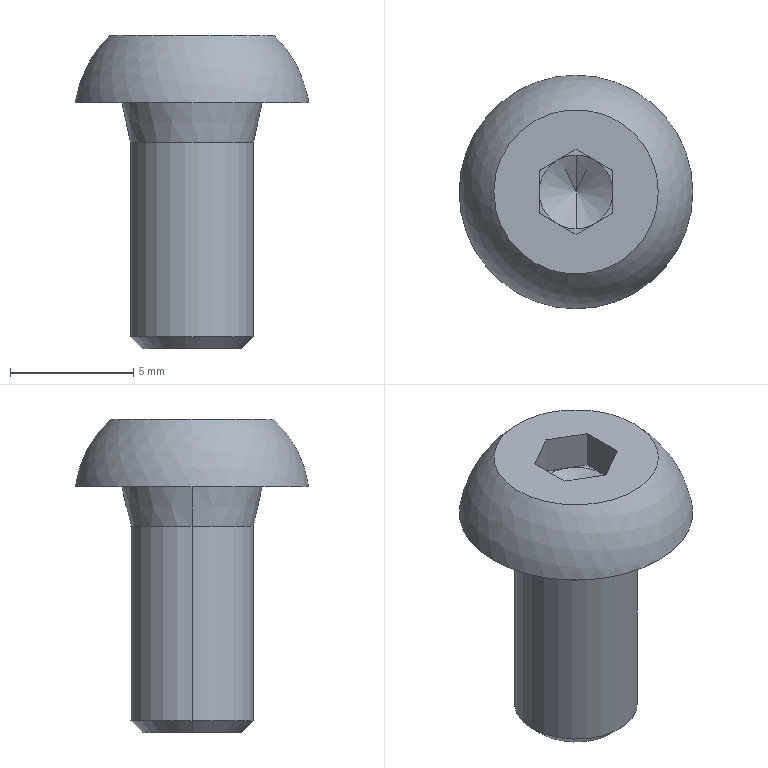Part | SolidWorks | features BaseBody 1 | 1 solid | 24 faces | box 9.5 x 9.5 x 12.75 mm | volume 341.504 mm3 | plane 15 | cone 6 | cylinder 2 | sphere 1 | commonest cylinder face diameters 5 x2
STEP:
#1=CARTESIAN_POINT('',(2.5,0.,0.));
#2=VERTEX_POINT('',#1);
#3=CARTESIAN_POINT('',(-2.5,0.,0.));
#4=VERTEX_POINT('',#3);
#5=CARTESIAN_POINT('',(0.,0.,0.));
#6=DIRECTION('',(0.,0.,1.));
#7=DIRECTION('',(1.,0.,0.));
#8=AXIS2_PLACEMENT_3D('',#5,#6,#7);
#9=CIRCLE('',#8,2.5);
#10=EDGE_CURVE('',#2,#4,#9,.T.);
#11=ORIENTED_EDGE('',*,*,#10,.T.);
#12=CARTESIAN_POINT('',(-2.85,0.,1.6));
#13=VERTEX_POINT('',#12);
#14=CARTESIAN_POINT('',(-2.85,0.,1.6));
#15=DIRECTION('',(-0.2137,0.,0.9769));
#16=VECTOR('',#15,1000.);
#17=LINE('',#14,#16);
#18=EDGE_CURVE('',#4,#13,#17,.T.);
#19=ORIENTED_EDGE('',*,*,#18,.T.);
#20=CARTESIAN_POINT('',(2.85,0.,1.6));
#21=VERTEX_POINT('',#20);
#22=CARTESIAN_POINT('',(0.,0.,1.6));
#23=DIRECTION('',(0.,0.,-1.));
#24=DIRECTION('',(1.,0.,0.));
#25=AXIS2_PLACEMENT_3D('',#22,#23,#24);
#26=CIRCLE('',#25,2.85);
#27=EDGE_CURVE('',#13,#21,#26,.T.);
#28=ORIENTED_EDGE('',*,*,#27,.T.);
#29=CARTESIAN_POINT('',(2.85,0.,1.6));
#30=DIRECTION('',(0.2137,0.,0.9769));
#31=VECTOR('',#30,1000.);
#32=LINE('',#29,#31);
#33=EDGE_CURVE('',#2,#21,#32,.T.);
#34=ORIENTED_EDGE('',*,*,#33,.F.);
#35=EDGE_LOOP('',(#11,#19,#28,#34));
#36=FACE_OUTER_BOUND('',#35,.T.);
#37=CARTESIAN_POINT('',(0.,0.,1.6));
#38=DIRECTION('',(0.,0.,1.));
#39=DIRECTION('',(1.,0.,0.));
#40=AXIS2_PLACEMENT_3D('',#37,#38,#39);
#41=CONICAL_SURFACE('',#40,2.85,0.2154);
#42=ADVANCED_FACE('',(#36),#41,.T.);
#43=CARTESIAN_POINT('',(2.5,0.,-7.91));
#44=VERTEX_POINT('',#43);
#45=CARTESIAN_POINT('',(-2.5,0.,-7.91));
#46=VERTEX_POINT('',#45);
#47=CARTESIAN_POINT('',(0.,0.,-7.91));
#48=DIRECTION('',(0.,0.,1.));
#49=DIRECTION('',(1.,0.,0.));
#50=AXIS2_PLACEMENT_3D('',#47,#48,#49);
#51=CIRCLE('',#50,2.5);
#52=EDGE_CURVE('',#44,#46,#51,.T.);
#53=ORIENTED_EDGE('',*,*,#52,.T.);
#54=CARTESIAN_POINT('',(-2.5,0.,-8.4));
#55=DIRECTION('',(0.,0.,1.));
#56=VECTOR('',#55,1000.);
#57=LINE('',#54,#56);
#58=EDGE_CURVE('',#46,#4,#57,.T.);
#59=ORIENTED_EDGE('',*,*,#58,.T.);
#60=ORIENTED_EDGE('',*,*,#10,.F.);
#61=CARTESIAN_POINT('',(2.5,0.,-8.4));
#62=DIRECTION('',(0.,0.,1.));
#63=VECTOR('',#62,1000.);
#64=LINE('',#61,#63);
#65=EDGE_CURVE('',#44,#2,#64,.T.);
#66=ORIENTED_EDGE('',*,*,#65,.F.);
#67=EDGE_LOOP('',(#53,#59,#60,#66));
#68=FACE_OUTER_BOUND('',#67,.T.);
#69=CARTESIAN_POINT('',(0.,0.,-8.4));
#70=DIRECTION('',(0.,0.,1.));
#71=DIRECTION('',(1.,0.,0.));
#72=AXIS2_PLACEMENT_3D('',#69,#70,#71);
#73=CYLINDRICAL_SURFACE('',#72,2.5);
#74=ADVANCED_FACE('',(#68),#73,.T.);
#75=CARTESIAN_POINT('',(0.,0.,1.924));
#76=VERTEX_POINT('',#75);
#77=CARTESIAN_POINT('',(0.,-1.5,2.79));
#78=VERTEX_POINT('',#77);
#79=CARTESIAN_POINT('',(0.,-1.5,2.79));
#80=DIRECTION('',(0.,-0.866,0.5));
#81=VECTOR('',#80,1000.);
#82=LINE('',#79,#81);
#83=EDGE_CURVE('',#76,#78,#82,.T.);
#84=ORIENTED_EDGE('',*,*,#83,.F.);
#85=CARTESIAN_POINT('',(0.,1.5,2.79));
#86=VERTEX_POINT('',#85);
#87=CARTESIAN_POINT('',(0.,1.5,2.79));
#88=DIRECTION('',(0.,0.866,0.5));
#89=VECTOR('',#88,1000.);
#90=LINE('',#87,#89);
#91=EDGE_CURVE('',#76,#86,#90,.T.);
#92=ORIENTED_EDGE('',*,*,#91,.T.);
#93=CARTESIAN_POINT('',(-0.75,1.299,2.79));
#94=VERTEX_POINT('',#93);
#95=CARTESIAN_POINT('',(0.,0.,2.79));
#96=DIRECTION('',(0.,0.,-1.));
#97=DIRECTION('',(0.,-1.,0.));
#98=AXIS2_PLACEMENT_3D('',#95,#96,#97);
#99=CIRCLE('',#98,1.5);
#100=EDGE_CURVE('',#94,#86,#99,.T.);
#101=ORIENTED_EDGE('',*,*,#100,.F.);
#102=CARTESIAN_POINT('',(-1.5,0.,2.79));
#103=VERTEX_POINT('',#102);
#104=CARTESIAN_POINT('',(0.,0.,2.79));
#105=DIRECTION('',(0.,0.,-1.));
#106=DIRECTION('',(0.,-1.,0.));
#107=AXIS2_PLACEMENT_3D('',#104,#105,#106);
#108=CIRCLE('',#107,1.5);
#109=EDGE_CURVE('',#103,#94,#108,.T.);
#110=ORIENTED_EDGE('',*,*,#109,.F.);
#111=CARTESIAN_POINT('',(-0.75,-1.299,2.79));
#112=VERTEX_POINT('',#111);
#113=CARTESIAN_POINT('',(0.,0.,2.79));
#114=DIRECTION('',(0.,0.,-1.));
#115=DIRECTION('',(0.,-1.,0.));
#116=AXIS2_PLACEMENT_3D('',#113,#114,#115);
#117=CIRCLE('',#116,1.5);
#118=EDGE_CURVE('',#112,#103,#117,.T.);
#119=ORIENTED_EDGE('',*,*,#118,.F.);
#120=CARTESIAN_POINT('',(0.,0.,2.79));
#121=DIRECTION('',(0.,0.,-1.));
#122=DIRECTION('',(0.,-1.,0.));
#123=AXIS2_PLACEMENT_3D('',#120,#121,#122);
#124=CIRCLE('',#123,1.5);
#125=EDGE_CURVE('',#78,#112,#124,.T.);
#126=ORIENTED_EDGE('',*,*,#125,.F.);
#127=EDGE_LOOP('',(#84,#92,#101,#110,#119,#126));
#128=FACE_OUTER_BOUND('',#127,.T.);
#129=CARTESIAN_POINT('',(0.,0.,2.79));
#130=DIRECTION('',(0.,0.,1.));
#131=DIRECTION('',(0.,-1.,0.));
#132=AXIS2_PLACEMENT_3D('',#129,#130,#131);
#133=CONICAL_SURFACE('',#132,1.5,1.047);
#134=ADVANCED_FACE('',(#128),#133,.F.);
#135=CARTESIAN_POINT('',(2.01,0.,-8.4));
#136=VERTEX_POINT('',#135);
#137=CARTESIAN_POINT('',(-2.01,0.,-8.4));
#138=VERTEX_POINT('',#137);
#139=CARTESIAN_POINT('',(0.,0.,-8.4));
#140=DIRECTION('',(0.,0.,1.));
#141=DIRECTION('',(1.,0.,0.));
#142=AXIS2_PLACEMENT_3D('',#139,#140,#141);
#143=CIRCLE('',#142,2.01);
#144=EDGE_CURVE('',#136,#138,#143,.T.);
#145=ORIENTED_EDGE('',*,*,#144,.T.);
#146=CARTESIAN_POINT('',(-2.5,0.,-7.91));
#147=DIRECTION('',(-0.7071,0.,0.7071));
#148=VECTOR('',#147,1000.);
#149=LINE('',#146,#148);
#150=EDGE_CURVE('',#138,#46,#149,.T.);
#151=ORIENTED_EDGE('',*,*,#150,.T.);
#152=ORIENTED_EDGE('',*,*,#52,.F.);
#153=CARTESIAN_POINT('',(2.5,0.,-7.91));
#154=DIRECTION('',(0.7071,0.,0.7071));
#155=VECTOR('',#154,1000.);
#156=LINE('',#153,#155);
#157=EDGE_CURVE('',#136,#44,#156,.T.);
#158=ORIENTED_EDGE('',*,*,#157,.F.);
#159=EDGE_LOOP('',(#145,#151,#152,#158));
#160=FACE_OUTER_BOUND('',#159,.T.);
#161=CARTESIAN_POINT('',(0.,0.,-7.91));
#162=DIRECTION('',(0.,0.,1.));
#163=DIRECTION('',(1.,0.,0.));
#164=AXIS2_PLACEMENT_3D('',#161,#162,#163);
#165=CONICAL_SURFACE('',#164,2.5,0.7854);
#166=ADVANCED_FACE('',(#160),#165,.T.);
#167=CARTESIAN_POINT('',(-3.339,0.,4.35));
#168=VERTEX_POINT('',#167);
#169=CARTESIAN_POINT('',(3.339,0.,4.35));
#170=VERTEX_POINT('',#169);
#171=CARTESIAN_POINT('',(0.,0.,4.35));
#172=DIRECTION('',(0.,0.,-1.));
#173=DIRECTION('',(-1.,0.,0.));
#174=AXIS2_PLACEMENT_3D('',#171,#172,#173);
#175=CIRCLE('',#174,3.339);
#176=EDGE_CURVE('',#168,#170,#175,.T.);
#177=ORIENTED_EDGE('',*,*,#176,.T.);
#178=CARTESIAN_POINT('',(0.,0.,4.35));
#179=DIRECTION('',(0.,0.,-1.));
#180=DIRECTION('',(-1.,0.,0.));
#181=AXIS2_PLACEMENT_3D('',#178,#179,#180);
#182=CIRCLE('',#181,3.339);
#183=EDGE_CURVE('',#170,#168,#182,.T.);
#184=ORIENTED_EDGE('',*,*,#183,.T.);
#185=EDGE_LOOP('',(#177,#184));
#186=FACE_BOUND('',#185,.T.);
#187=CARTESIAN_POINT('',(4.75,0.,1.6));
#188=VERTEX_POINT('',#187);
#189=CARTESIAN_POINT('',(-4.75,0.,1.6));
#190=VERTEX_POINT('',#189);
#191=CARTESIAN_POINT('',(0.,0.,1.6));
#192=DIRECTION('',(0.,0.,1.));
#193=DIRECTION('',(1.,0.,0.));
#194=AXIS2_PLACEMENT_3D('',#191,#192,#193);
#195=CIRCLE('',#194,4.75);
#196=EDGE_CURVE('',#188,#190,#195,.T.);
#197=ORIENTED_EDGE('',*,*,#196,.T.);
#198=CARTESIAN_POINT('',(0.,0.,1.6));
#199=DIRECTION('',(0.,0.,1.));
#200=DIRECTION('',(1.,0.,0.));
#201=AXIS2_PLACEMENT_3D('',#198,#199,#200);
#202=CIRCLE('',#201,4.75);
#203=EDGE_CURVE('',#190,#188,#202,.T.);
#204=ORIENTED_EDGE('',*,*,#203,.T.);
#205=EDGE_LOOP('',(#197,#204));
#206=FACE_OUTER_BOUND('',#205,.T.);
#207=CARTESIAN_POINT('',(0.,0.,0.9));
#208=DIRECTION('',(0.1289,0.,0.9917));
#209=DIRECTION('',(-0.9917,0.,0.1289));
#210=AXIS2_PLACEMENT_3D('',#207,#208,#209);
#211=SPHERICAL_SURFACE('',#210,4.801);
#212=ADVANCED_FACE('',(#186,#206),#211,.T.);
#213=ORIENTED_EDGE('',*,*,#176,.F.);
#214=ORIENTED_EDGE('',*,*,#183,.F.);
#215=EDGE_LOOP('',(#213,#214));
#216=FACE_OUTER_BOUND('',#215,.T.);
#217=CARTESIAN_POINT('',(0.,-1.732,4.35));
#218=VERTEX_POINT('',#217);
#219=CARTESIAN_POINT('',(1.5,-0.866,4.35));
#220=VERTEX_POINT('',#219);
#221=CARTESIAN_POINT('',(0.,-1.732,4.35));
#222=DIRECTION('',(0.866,0.5,0.));
#223=VECTOR('',#222,1000.);
#224=LINE('',#221,#223);
#225=EDGE_CURVE('',#218,#220,#224,.T.);
#226=ORIENTED_EDGE('',*,*,#225,.F.);
#227=CARTESIAN_POINT('',(-1.5,-0.866,4.35));
#228=VERTEX_POINT('',#227);
#229=CARTESIAN_POINT('',(-1.5,-0.866,4.35));
#230=DIRECTION('',(0.866,-0.5,0.));
#231=VECTOR('',#230,1000.);
#232=LINE('',#229,#231);
#233=EDGE_CURVE('',#228,#218,#232,.T.);
#234=ORIENTED_EDGE('',*,*,#233,.F.);
#235=CARTESIAN_POINT('',(-1.5,0.866,4.35));
#236=VERTEX_POINT('',#235);
#237=CARTESIAN_POINT('',(-1.5,0.,4.35));
#238=DIRECTION('',(0.,-1.,0.));
#239=VECTOR('',#238,1000.);
#240=LINE('',#237,#239);
#241=EDGE_CURVE('',#236,#228,#240,.T.);
#242=ORIENTED_EDGE('',*,*,#241,.F.);
#243=CARTESIAN_POINT('',(0.,1.732,4.35));
#244=VERTEX_POINT('',#243);
#245=CARTESIAN_POINT('',(0.,1.732,4.35));
#246=DIRECTION('',(-0.866,-0.5,0.));
#247=VECTOR('',#246,1000.);
#248=LINE('',#245,#247);
#249=EDGE_CURVE('',#244,#236,#248,.T.);
#250=ORIENTED_EDGE('',*,*,#249,.F.);
#251=CARTESIAN_POINT('',(1.5,0.866,4.35));
#252=VERTEX_POINT('',#251);
#253=CARTESIAN_POINT('',(1.5,0.866,4.35));
#254=DIRECTION('',(-0.866,0.5,0.));
#255=VECTOR('',#254,1000.);
#256=LINE('',#253,#255);
#257=EDGE_CURVE('',#252,#244,#256,.T.);
#258=ORIENTED_EDGE('',*,*,#257,.F.);
#259=CARTESIAN_POINT('',(1.5,0.,4.35));
#260=DIRECTION('',(0.,1.,0.));
#261=VECTOR('',#260,1000.);
#262=LINE('',#259,#261);
#263=EDGE_CURVE('',#220,#252,#262,.T.);
#264=ORIENTED_EDGE('',*,*,#263,.F.);
#265=EDGE_LOOP('',(#226,#234,#242,#250,#258,#264));
#266=FACE_BOUND('',#265,.T.);
#267=CARTESIAN_POINT('',(0.,0.,4.35));
#268=DIRECTION('',(0.,0.,-1.));
#269=DIRECTION('',(-1.,0.,0.));
#270=AXIS2_PLACEMENT_3D('',#267,#268,#269);
#271=PLANE('',#270);
#272=ADVANCED_FACE('',(#216,#266),#271,.F.);
#273=ORIENTED_EDGE('',*,*,#196,.F.);
#274=ORIENTED_EDGE('',*,*,#203,.F.);
#275=EDGE_LOOP('',(#273,#274));
#276=FACE_OUTER_BOUND('',#275,.T.);
#277=CARTESIAN_POINT('',(0.,0.,1.6));
#278=DIRECTION('',(0.,0.,-1.));
#279=DIRECTION('',(1.,0.,0.));
#280=AXIS2_PLACEMENT_3D('',#277,#278,#279);
#281=CIRCLE('',#280,2.85);
#282=EDGE_CURVE('',#21,#13,#281,.T.);
#283=ORIENTED_EDGE('',*,*,#282,.F.);
#284=ORIENTED_EDGE('',*,*,#27,.F.);
#285=EDGE_LOOP('',(#283,#284));
#286=FACE_BOUND('',#285,.T.);
#287=CARTESIAN_POINT('',(0.,4.75,1.6));
#288=DIRECTION('',(0.,0.,1.));
#289=DIRECTION('',(1.,0.,0.));
#290=AXIS2_PLACEMENT_3D('',#287,#288,#289);
#291=PLANE('',#290);
#292=ADVANCED_FACE('',(#276,#286),#291,.F.);
#293=CARTESIAN_POINT('',(1.5,0.866,2.79));
#294=VERTEX_POINT('',#293);
#295=CARTESIAN_POINT('',(1.5,0.866,2.79));
#296=DIRECTION('',(0.,0.,1.));
#297=VECTOR('',#296,1000.);
#298=LINE('',#295,#297);
#299=EDGE_CURVE('',#294,#252,#298,.T.);
#300=ORIENTED_EDGE('',*,*,#299,.F.);
#301=CARTESIAN_POINT('',(1.5,0.,2.79));
#302=VERTEX_POINT('',#301);
#303=CARTESIAN_POINT('',(1.5,-0.866,2.79));
#304=DIRECTION('',(0.,1.,0.));
#305=VECTOR('',#304,1000.);
#306=LINE('',#303,#305);
#307=EDGE_CURVE('',#302,#294,#306,.T.);
#308=ORIENTED_EDGE('',*,*,#307,.F.);
#309=CARTESIAN_POINT('',(1.5,-0.866,2.79));
#310=VERTEX_POINT('',#309);
#311=CARTESIAN_POINT('',(1.5,-0.866,2.79));
#312=DIRECTION('',(0.,1.,0.));
#313=VECTOR('',#312,1000.);
#314=LINE('',#311,#313);
#315=EDGE_CURVE('',#310,#302,#314,.T.);
#316=ORIENTED_EDGE('',*,*,#315,.F.);
#317=CARTESIAN_POINT('',(1.5,-0.866,2.79));
#318=DIRECTION('',(0.,0.,-1.));
#319=VECTOR('',#318,1000.);
#320=LINE('',#317,#319);
#321=EDGE_CURVE('',#220,#310,#320,.T.);
#322=ORIENTED_EDGE('',*,*,#321,.F.);
#323=ORIENTED_EDGE('',*,*,#263,.T.);
#324=EDGE_LOOP('',(#300,#308,#316,#322,#323));
#325=FACE_OUTER_BOUND('',#324,.T.);
#326=CARTESIAN_POINT('',(1.5,-0.866,2.79));
#327=DIRECTION('',(1.,0.,0.));
#328=DIRECTION('',(0.,0.,-1.));
#329=AXIS2_PLACEMENT_3D('',#326,#327,#328);
#330=PLANE('',#329);
#331=ADVANCED_FACE('',(#325),#330,.F.);
#332=ORIENTED_EDGE('',*,*,#321,.T.);
#333=CARTESIAN_POINT('',(0.75,-1.299,2.79));
#334=VERTEX_POINT('',#333);
#335=CARTESIAN_POINT('',(0.,-1.732,2.79));
#336=DIRECTION('',(0.866,0.5,0.));
#337=VECTOR('',#336,1000.);
#338=LINE('',#335,#337);
#339=EDGE_CURVE('',#334,#310,#338,.T.);
#340=ORIENTED_EDGE('',*,*,#339,.F.);
#341=CARTESIAN_POINT('',(0.,-1.732,2.79));
#342=VERTEX_POINT('',#341);
#343=CARTESIAN_POINT('',(0.,-1.732,2.79));
#344=DIRECTION('',(0.866,0.5,0.));
#345=VECTOR('',#344,1000.);
#346=LINE('',#343,#345);
#347=EDGE_CURVE('',#342,#334,#346,.T.);
#348=ORIENTED_EDGE('',*,*,#347,.F.);
#349=CARTESIAN_POINT('',(0.,-1.732,2.79));
#350=DIRECTION('',(0.,0.,-1.));
#351=VECTOR('',#350,1000.);
#352=LINE('',#349,#351);
#353=EDGE_CURVE('',#218,#342,#352,.T.);
#354=ORIENTED_EDGE('',*,*,#353,.F.);
#355=ORIENTED_EDGE('',*,*,#225,.T.);
#356=EDGE_LOOP('',(#332,#340,#348,#354,#355));
#357=FACE_OUTER_BOUND('',#356,.T.);
#358=CARTESIAN_POINT('',(0.,-1.732,2.79));
#359=DIRECTION('',(0.5,-0.866,0.));
#360=DIRECTION('',(0.866,0.5,0.));
#361=AXIS2_PLACEMENT_3D('',#358,#359,#360);
#362=PLANE('',#361);
#363=ADVANCED_FACE('',(#357),#362,.F.);
#364=ORIENTED_EDGE('',*,*,#353,.T.);
#365=CARTESIAN_POINT('',(-1.5,-0.866,2.79));
#366=DIRECTION('',(0.866,-0.5,0.));
#367=VECTOR('',#366,1000.);
#368=LINE('',#365,#367);
#369=EDGE_CURVE('',#112,#342,#368,.T.);
#370=ORIENTED_EDGE('',*,*,#369,.F.);
#371=CARTESIAN_POINT('',(-1.5,-0.866,2.79));
#372=VERTEX_POINT('',#371);
#373=CARTESIAN_POINT('',(-1.5,-0.866,2.79));
#374=DIRECTION('',(0.866,-0.5,0.));
#375=VECTOR('',#374,1000.);
#376=LINE('',#373,#375);
#377=EDGE_CURVE('',#372,#112,#376,.T.);
#378=ORIENTED_EDGE('',*,*,#377,.F.);
#379=CARTESIAN_POINT('',(-1.5,-0.866,2.79));
#380=DIRECTION('',(0.,0.,-1.));
#381=VECTOR('',#380,1000.);
#382=LINE('',#379,#381);
#383=EDGE_CURVE('',#228,#372,#382,.T.);
#384=ORIENTED_EDGE('',*,*,#383,.F.);
#385=ORIENTED_EDGE('',*,*,#233,.T.);
#386=EDGE_LOOP('',(#364,#370,#378,#384,#385));
#387=FACE_OUTER_BOUND('',#386,.T.);
#388=CARTESIAN_POINT('',(-1.5,-0.866,2.79));
#389=DIRECTION('',(-0.5,-0.866,0.));
#390=DIRECTION('',(0.866,-0.5,0.));
#391=AXIS2_PLACEMENT_3D('',#388,#389,#390);
#392=PLANE('',#391);
#393=ADVANCED_FACE('',(#387),#392,.F.);
#394=ORIENTED_EDGE('',*,*,#383,.T.);
#395=CARTESIAN_POINT('',(-1.5,0.866,2.79));
#396=DIRECTION('',(0.,-1.,0.));
#397=VECTOR('',#396,1000.);
#398=LINE('',#395,#397);
#399=EDGE_CURVE('',#103,#372,#398,.T.);
#400=ORIENTED_EDGE('',*,*,#399,.F.);
#401=CARTESIAN_POINT('',(-1.5,0.866,2.79));
#402=VERTEX_POINT('',#401);
#403=CARTESIAN_POINT('',(-1.5,0.866,2.79));
#404=DIRECTION('',(0.,-1.,0.));
#405=VECTOR('',#404,1000.);
#406=LINE('',#403,#405);
#407=EDGE_CURVE('',#402,#103,#406,.T.);
#408=ORIENTED_EDGE('',*,*,#407,.F.);
#409=CARTESIAN_POINT('',(-1.5,0.866,2.79));
#410=DIRECTION('',(0.,0.,-1.));
#411=VECTOR('',#410,1000.);
#412=LINE('',#409,#411);
#413=EDGE_CURVE('',#236,#402,#412,.T.);
#414=ORIENTED_EDGE('',*,*,#413,.F.);
#415=ORIENTED_EDGE('',*,*,#241,.T.);
#416=EDGE_LOOP('',(#394,#400,#408,#414,#415));
#417=FACE_OUTER_BOUND('',#416,.T.);
#418=CARTESIAN_POINT('',(-1.5,0.866,2.79));
#419=DIRECTION('',(-1.,0.,0.));
#420=DIRECTION('',(0.,-1.,0.));
#421=AXIS2_PLACEMENT_3D('',#418,#419,#420);
#422=PLANE('',#421);
#423=ADVANCED_FACE('',(#417),#422,.F.);
#424=ORIENTED_EDGE('',*,*,#413,.T.);
#425=CARTESIAN_POINT('',(0.,1.732,2.79));
#426=DIRECTION('',(-0.866,-0.5,0.));
#427=VECTOR('',#426,1000.);
#428=LINE('',#425,#427);
#429=EDGE_CURVE('',#94,#402,#428,.T.);
#430=ORIENTED_EDGE('',*,*,#429,.F.);
#431=CARTESIAN_POINT('',(0.,1.732,2.79));
#432=VERTEX_POINT('',#431);
#433=CARTESIAN_POINT('',(0.,1.732,2.79));
#434=DIRECTION('',(-0.866,-0.5,0.));
#435=VECTOR('',#434,1000.);
#436=LINE('',#433,#435);
#437=EDGE_CURVE('',#432,#94,#436,.T.);
#438=ORIENTED_EDGE('',*,*,#437,.F.);
#439=CARTESIAN_POINT('',(0.,1.732,2.79));
#440=DIRECTION('',(0.,0.,-1.));
#441=VECTOR('',#440,1000.);
#442=LINE('',#439,#441);
#443=EDGE_CURVE('',#244,#432,#442,.T.);
#444=ORIENTED_EDGE('',*,*,#443,.F.);
#445=ORIENTED_EDGE('',*,*,#249,.T.);
#446=EDGE_LOOP('',(#424,#430,#438,#444,#445));
#447=FACE_OUTER_BOUND('',#446,.T.);
#448=CARTESIAN_POINT('',(0.,1.732,2.79));
#449=DIRECTION('',(-0.5,0.866,0.));
#450=DIRECTION('',(-0.866,-0.5,0.));
#451=AXIS2_PLACEMENT_3D('',#448,#449,#450);
#452=PLANE('',#451);
#453=ADVANCED_FACE('',(#447),#452,.F.);
#454=ORIENTED_EDGE('',*,*,#443,.T.);
#455=CARTESIAN_POINT('',(0.75,1.299,2.79));
#456=VERTEX_POINT('',#455);
#457=CARTESIAN_POINT('',(1.5,0.866,2.79));
#458=DIRECTION('',(-0.866,0.5,0.));
#459=VECTOR('',#458,1000.);
#460=LINE('',#457,#459);
#461=EDGE_CURVE('',#456,#432,#460,.T.);
#462=ORIENTED_EDGE('',*,*,#461,.F.);
#463=CARTESIAN_POINT('',(1.5,0.866,2.79));
#464=DIRECTION('',(-0.866,0.5,0.));
#465=VECTOR('',#464,1000.);
#466=LINE('',#463,#465);
#467=EDGE_CURVE('',#294,#456,#466,.T.);
#468=ORIENTED_EDGE('',*,*,#467,.F.);
#469=ORIENTED_EDGE('',*,*,#299,.T.);
#470=ORIENTED_EDGE('',*,*,#257,.T.);
#471=EDGE_LOOP('',(#454,#462,#468,#469,#470));
#472=FACE_OUTER_BOUND('',#471,.T.);
#473=CARTESIAN_POINT('',(1.5,0.866,2.79));
#474=DIRECTION('',(0.5,0.866,0.));
#475=DIRECTION('',(-0.866,0.5,0.));
#476=AXIS2_PLACEMENT_3D('',#473,#474,#475);
#477=PLANE('',#476);
#478=ADVANCED_FACE('',(#472),#477,.F.);
#479=ORIENTED_EDGE('',*,*,#18,.F.);
#480=CARTESIAN_POINT('',(0.,0.,0.));
#481=DIRECTION('',(0.,0.,1.));
#482=DIRECTION('',(1.,0.,0.));
#483=AXIS2_PLACEMENT_3D('',#480,#481,#482);
#484=CIRCLE('',#483,2.5);
#485=EDGE_CURVE('',#4,#2,#484,.T.);
#486=ORIENTED_EDGE('',*,*,#485,.T.);
#487=ORIENTED_EDGE('',*,*,#33,.T.);
#488=ORIENTED_EDGE('',*,*,#282,.T.);
#489=EDGE_LOOP('',(#479,#486,#487,#488));
#490=FACE_OUTER_BOUND('',#489,.T.);
#491=CARTESIAN_POINT('',(0.,0.,1.6));
#492=DIRECTION('',(0.,0.,1.));
#493=DIRECTION('',(1.,0.,0.));
#494=AXIS2_PLACEMENT_3D('',#491,#492,#493);
#495=CONICAL_SURFACE('',#494,2.85,0.2154);
#496=ADVANCED_FACE('',(#490),#495,.T.);
#497=CARTESIAN_POINT('',(0.,0.,2.79));
#498=DIRECTION('',(0.,0.,-1.));
#499=DIRECTION('',(0.,-1.,0.));
#500=AXIS2_PLACEMENT_3D('',#497,#498,#499);
#501=CIRCLE('',#500,1.5);
#502=EDGE_CURVE('',#456,#302,#501,.T.);
#503=ORIENTED_EDGE('',*,*,#502,.T.);
#504=ORIENTED_EDGE('',*,*,#307,.T.);
#505=ORIENTED_EDGE('',*,*,#467,.T.);
#506=EDGE_LOOP('',(#503,#504,#505));
#507=FACE_OUTER_BOUND('',#506,.T.);
#508=CARTESIAN_POINT('',(0.,0.,2.79));
#509=DIRECTION('',(0.,0.,1.));
#510=DIRECTION('',(1.,0.,0.));
#511=AXIS2_PLACEMENT_3D('',#508,#509,#510);
#512=PLANE('',#511);
#513=ADVANCED_FACE('',(#507),#512,.T.);
#514=CARTESIAN_POINT('',(0.,0.,2.79));
#515=DIRECTION('',(0.,0.,-1.));
#516=DIRECTION('',(0.,-1.,0.));
#517=AXIS2_PLACEMENT_3D('',#514,#515,#516);
#518=CIRCLE('',#517,1.5);
#519=EDGE_CURVE('',#302,#334,#518,.T.);
#520=ORIENTED_EDGE('',*,*,#519,.T.);
#521=ORIENTED_EDGE('',*,*,#339,.T.);
#522=ORIENTED_EDGE('',*,*,#315,.T.);
#523=EDGE_LOOP('',(#520,#521,#522));
#524=FACE_OUTER_BOUND('',#523,.T.);
#525=CARTESIAN_POINT('',(0.,0.,2.79));
#526=DIRECTION('',(0.,0.,1.));
#527=DIRECTION('',(1.,0.,0.));
#528=AXIS2_PLACEMENT_3D('',#525,#526,#527);
#529=PLANE('',#528);
#530=ADVANCED_FACE('',(#524),#529,.T.);
#531=CARTESIAN_POINT('',(0.,0.,2.79));
#532=DIRECTION('',(0.,0.,-1.));
#533=DIRECTION('',(0.,-1.,0.));
#534=AXIS2_PLACEMENT_3D('',#531,#532,#533);
#535=CIRCLE('',#534,1.5);
#536=EDGE_CURVE('',#334,#78,#535,.T.);
#537=ORIENTED_EDGE('',*,*,#536,.T.);
#538=ORIENTED_EDGE('',*,*,#125,.T.);
#539=ORIENTED_EDGE('',*,*,#369,.T.);
#540=ORIENTED_EDGE('',*,*,#347,.T.);
#541=EDGE_LOOP('',(#537,#538,#539,#540));
#542=FACE_OUTER_BOUND('',#541,.T.);
#543=CARTESIAN_POINT('',(0.,0.,2.79));
#544=DIRECTION('',(0.,0.,1.));
#545=DIRECTION('',(1.,0.,0.));
#546=AXIS2_PLACEMENT_3D('',#543,#544,#545);
#547=PLANE('',#546);
#548=ADVANCED_FACE('',(#542),#547,.T.);
#549=ORIENTED_EDGE('',*,*,#118,.T.);
#550=ORIENTED_EDGE('',*,*,#399,.T.);
#551=ORIENTED_EDGE('',*,*,#377,.T.);
#552=EDGE_LOOP('',(#549,#550,#551));
#553=FACE_OUTER_BOUND('',#552,.T.);
#554=CARTESIAN_POINT('',(0.,0.,2.79));
#555=DIRECTION('',(0.,0.,1.));
#556=DIRECTION('',(1.,0.,0.));
#557=AXIS2_PLACEMENT_3D('',#554,#555,#556);
#558=PLANE('',#557);
#559=ADVANCED_FACE('',(#553),#558,.T.);
#560=ORIENTED_EDGE('',*,*,#109,.T.);
#561=ORIENTED_EDGE('',*,*,#429,.T.);
#562=ORIENTED_EDGE('',*,*,#407,.T.);
#563=EDGE_LOOP('',(#560,#561,#562));
#564=FACE_OUTER_BOUND('',#563,.T.);
#565=CARTESIAN_POINT('',(0.,0.,2.79));
#566=DIRECTION('',(0.,0.,1.));
#567=DIRECTION('',(1.,0.,0.));
#568=AXIS2_PLACEMENT_3D('',#565,#566,#567);
#569=PLANE('',#568);
#570=ADVANCED_FACE('',(#564),#569,.T.);
#571=ORIENTED_EDGE('',*,*,#100,.T.);
#572=CARTESIAN_POINT('',(0.,0.,2.79));
#573=DIRECTION('',(0.,0.,-1.));
#574=DIRECTION('',(0.,-1.,0.));
#575=AXIS2_PLACEMENT_3D('',#572,#573,#574);
#576=CIRCLE('',#575,1.5);
#577=EDGE_CURVE('',#86,#456,#576,.T.);
#578=ORIENTED_EDGE('',*,*,#577,.T.);
#579=ORIENTED_EDGE('',*,*,#461,.T.);
#580=ORIENTED_EDGE('',*,*,#437,.T.);
#581=EDGE_LOOP('',(#571,#578,#579,#580));
#582=FACE_OUTER_BOUND('',#581,.T.);
#583=CARTESIAN_POINT('',(0.,0.,2.79));
#584=DIRECTION('',(0.,0.,1.));
#585=DIRECTION('',(1.,0.,0.));
#586=AXIS2_PLACEMENT_3D('',#583,#584,#585);
#587=PLANE('',#586);
#588=ADVANCED_FACE('',(#582),#587,.T.);
#589=ORIENTED_EDGE('',*,*,#58,.F.);
#590=CARTESIAN_POINT('',(0.,0.,-7.91));
#591=DIRECTION('',(0.,0.,1.));
#592=DIRECTION('',(1.,0.,0.));
#593=AXIS2_PLACEMENT_3D('',#590,#591,#592);
#594=CIRCLE('',#593,2.5);
#595=EDGE_CURVE('',#46,#44,#594,.T.);
#596=ORIENTED_EDGE('',*,*,#595,.T.);
#597=ORIENTED_EDGE('',*,*,#65,.T.);
#598=ORIENTED_EDGE('',*,*,#485,.F.);
#599=EDGE_LOOP('',(#589,#596,#597,#598));
#600=FACE_OUTER_BOUND('',#599,.T.);
#601=CARTESIAN_POINT('',(0.,0.,-8.4));
#602=DIRECTION('',(0.,0.,1.));
#603=DIRECTION('',(1.,0.,0.));
#604=AXIS2_PLACEMENT_3D('',#601,#602,#603);
#605=CYLINDRICAL_SURFACE('',#604,2.5);
#606=ADVANCED_FACE('',(#600),#605,.T.);
#607=ORIENTED_EDGE('',*,*,#91,.F.);
#608=ORIENTED_EDGE('',*,*,#83,.T.);
#609=ORIENTED_EDGE('',*,*,#536,.F.);
#610=ORIENTED_EDGE('',*,*,#519,.F.);
#611=ORIENTED_EDGE('',*,*,#502,.F.);
#612=ORIENTED_EDGE('',*,*,#577,.F.);
#613=EDGE_LOOP('',(#607,#608,#609,#610,#611,#612));
#614=FACE_OUTER_BOUND('',#613,.T.);
#615=CARTESIAN_POINT('',(0.,0.,2.79));
#616=DIRECTION('',(0.,0.,1.));
#617=DIRECTION('',(0.,-1.,0.));
#618=AXIS2_PLACEMENT_3D('',#615,#616,#617);
#619=CONICAL_SURFACE('',#618,1.5,1.047);
#620=ADVANCED_FACE('',(#614),#619,.F.);
#621=ORIENTED_EDGE('',*,*,#150,.F.);
#622=CARTESIAN_POINT('',(0.,0.,-8.4));
#623=DIRECTION('',(0.,0.,1.));
#624=DIRECTION('',(1.,0.,0.));
#625=AXIS2_PLACEMENT_3D('',#622,#623,#624);
#626=CIRCLE('',#625,2.01);
#627=EDGE_CURVE('',#138,#136,#626,.T.);
#628=ORIENTED_EDGE('',*,*,#627,.T.);
#629=ORIENTED_EDGE('',*,*,#157,.T.);
#630=ORIENTED_EDGE('',*,*,#595,.F.);
#631=EDGE_LOOP('',(#621,#628,#629,#630));
#632=FACE_OUTER_BOUND('',#631,.T.);
#633=CARTESIAN_POINT('',(0.,0.,-7.91));
#634=DIRECTION('',(0.,0.,1.));
#635=DIRECTION('',(1.,0.,0.));
#636=AXIS2_PLACEMENT_3D('',#633,#634,#635);
#637=CONICAL_SURFACE('',#636,2.5,0.7854);
#638=ADVANCED_FACE('',(#632),#637,.T.);
#639=ORIENTED_EDGE('',*,*,#144,.F.);
#640=ORIENTED_EDGE('',*,*,#627,.F.);
#641=EDGE_LOOP('',(#639,#640));
#642=FACE_OUTER_BOUND('',#641,.T.);
#643=CARTESIAN_POINT('',(2.5,0.,-8.4));
#644=DIRECTION('',(0.,0.,-1.));
#645=DIRECTION('',(-1.,0.,0.));
#646=AXIS2_PLACEMENT_3D('',#643,#644,#645);
#647=PLANE('',#646);
#648=ADVANCED_FACE('',(#642),#647,.T.);
#649=CLOSED_SHELL('',(#42,#74,#134,#166,#212,#272,#292,#331,#363,#393,#423,#453,#478,#496,#513,#530,#548,#559,#570,#588,#606,#620,#638,#648));
#650=MANIFOLD_SOLID_BREP('',#649);
#651=CARTESIAN_POINT('',(0.,0.,0.));
#652=DIRECTION('',(0.,0.,1.));
#653=DIRECTION('',(1.,0.,0.));
#654=AXIS2_PLACEMENT_3D('',#651,#652,#653);
#655=(LENGTH_UNIT()NAMED_UNIT(*)SI_UNIT(.MILLI.,.METRE.));
#656=UNCERTAINTY_MEASURE_WITH_UNIT(LENGTH_MEASURE(0.00001),#655,'','');
#657=(NAMED_UNIT(*)PLANE_ANGLE_UNIT()SI_UNIT($,.RADIAN.));
#658=(NAMED_UNIT(*)SI_UNIT($,.STERADIAN.)SOLID_ANGLE_UNIT());
#659=(GEOMETRIC_REPRESENTATION_CONTEXT(3)GLOBAL_UNCERTAINTY_ASSIGNED_CONTEXT((#656))GLOBAL_UNIT_ASSIGNED_CONTEXT((#655,#657,#658))REPRESENTATION_CONTEXT('',''));
#660=ADVANCED_BREP_SHAPE_REPRESENTATION('',(#650,#654),#659);